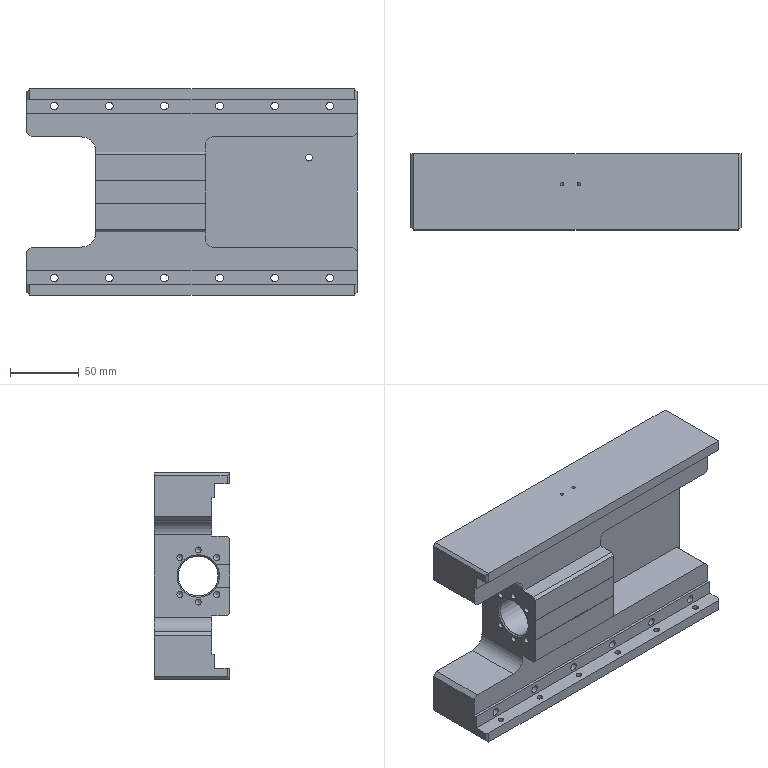CAM job | NX | 3+2 milling, drilling | part box 240 x 55 x 150 mm | stock box 245 x 60 x 155 mm
Tools:
number,name,description,diameter,corner_radius,flute_length,length,flutes
4,D4,平底铣刀-粗,4.0,0.0,25.0,75.0,2
6,D6,平底铣刀-粗,6.0,0.0,25.0,75.0,2
9,D10,平底铣刀-粗,10.0,0.0,35.0,75.0,2
17,D16,平底铣刀-粗,16.0,0.0,50.0,75.0,2
11,D4-J,平底铣刀-精,4.0,0.0,50.0,75.0,2
7,D6-J,平底铣刀-精,6.0,0.0,25.0,75.0,2
10,D10-J,平底铣刀-精,10.0,0.0,35.0,75.0,2
18,D16-J,平底铣刀-精,16.0,0.0,50.0,75.0,2
1,D80R0.8飞刀,圆鼻刀-粗,80.0,0.8,50.0,75.0,2
1,D80R0.8飞刀-J,圆鼻刀-精,80.0,0.8,50.0,75.0,2
2,D6倒角刀,倒角刀,6.0,0.0,3.0,25.0,2
19,D10倒角刀,倒角刀,10.0,0.0,5.0,75.0,2
21,M4X0.7,丝锥,3.3,0.0,35.0,50.0,2
22,M5X0.8,丝锥,4.2,0.0,35.0,50.0,2
23,M6X1.0,丝锥,5.0,0.0,35.0,50.0,2
15,ZT5,钻头,5.0,0.0,35.0,50.0,2
22,ZT5.5,钻头,5.5,0.0,35.0,50.0,2
18,ZT5.8,钻头,5.8,0.0,35.0,50.0,2
13,钻头3.3,Twist Drill 3.3 mm,3.3,0.0,35.0,35.008,2
14,钻头4.2,Twist Drill 4.2 mm,4.2,0.0,41.0,41.738,2
Operations:
program,operation,operation_type,tool,method,geometry_group,spindle_rpm,surface_speed,feed_per_tooth,feed_cut,feed_plunge,cut_length_mm,path_length_mm,cut_time_min,machine_time_min
C,等高往复层切开粗-中_COPY,ZLevelMilling,D16,分层开粗-切深K-步距G,W-C,4000.0,201.062,0.5,4000.0,100.0,13176.223,13478.223,3.294,3.324
C,打点-深0.8_2,Operation,D10倒角刀,NONE,W-C,5000.0,157.08,0.05,500.0,90.0,10.8,251.794,0.0216,0.0457
C,盲锥孔-M5螺纹底孔_2,Operation,钻头4.2,NONE,W-C,2500.0,32.987,0.03,150.0,90.0,87.971,406.136,0.5865,0.6183
C,铣倒角_6,PlanarMilling,D10倒角刀,METHOD,W-C,5000.0,157.08,0.05,500.0,100.0,86.111,1019.558,0.1722,0.2656
C,底壁铣倒角_COPY_1,VolumeBased25DMillingOperation,D10倒角刀,爬面_倒角-切深0-步距G,W-C,5000.0,157.08,0.1,1000.0,100.0,98.812,239.212,0.0988,0.1129
C,C0.3封闭铣廓倒角6X45L_COPY,PlanarMilling,D10倒角刀,爬面_倒角-切深0-步距G,W-C,5000.0,157.08,0.1,1000.0,100.0,45.144,335.469,0.0451,0.0742
C,底壁铣精光侧面-中_COPY,VolumeBased25DMillingOperation,D16-J,侧刃精光-切深K-步距G,W-C,3000.0,150.796,0.1667,1000.0,100.0,1007.169,1368.887,1.007,1.043
B,底壁铣飞面开粗_COPY,VolumeBased25DMillingOperation,D80R0.8飞刀,分层开粗-切深K-步距G,W-B,2800.0,703.696,0.5357,3000.0,100.0,9535.189,12950.012,3.178,3.52
B,底壁铣飞面精光_COPY,VolumeBased25DMillingOperation,D80R0.8飞刀-J,侧刃精光-切深K-步距G,W-B,4000.0,1005.28,0.125,1000.0,100.0,1058.658,1154.658,1.059,1.068
B,型腔铣开粗-中_COPY_1,CavityMilling,D10,分层开粗-切深K-步距G,W-B,8000.0,251.327,0.3125,5000.0,100.0,156407.598,167969.499,31.282,32.886
B,底壁铣精光底面-中_COPY,VolumeBased25DMillingOperation,D10-J,精光步距切深关,W-B,7000.0,175.0,0.0536,1500.0,100.0,3911.458,4582.386,2.608,2.675
B,底壁铣精光底面-中_COPY_1,VolumeBased25DMillingOperation,D10-J,精光步距切深关,W-B,7000.0,175.0,0.0536,1500.0,100.0,1585.376,1695.376,1.057,1.068
B,底壁铣精光侧面-中-选底面_COPY_1,VolumeBased25DMillingOperation,D10-J,侧刃精光-切深K-步距G,W-B,8000.0,251.32,0.0625,1000.0,100.0,712.444,972.215,0.7124,0.7384
B,底壁铣精光侧面-中-选底面_COPY_2,VolumeBased25DMillingOperation,D10-J,侧刃精光-切深K-步距G,W-B,8000.0,251.32,0.0625,1000.0,100.0,904.927,1155.753,0.9049,0.93
B,平面去毛刺6X45L_COPY,SurfaceContour,D6倒角刀,爬面_倒角-切深0-步距G,W-B,6500.0,122.519,0.1154,1500.0,100.0,2590.157,5472.976,1.727,2.015
B,底壁铣倒角_COPY,VolumeBased25DMillingOperation,D6倒角刀,爬面_倒角-切深0-步距G,W-B,6500.0,122.519,0.1154,1500.0,100.0,256.429,1478.093,0.171,0.2931
B,底壁铣精光侧面-中-选底面_COPY,VolumeBased25DMillingOperation,D10-J,侧刃精光-切深K-步距G,W-B,8000.0,251.32,0.0625,1000.0,100.0,516.566,711.587,0.5166,0.5361
A,顶面,FaceMilling,D80R0.8飞刀,侧刃精光-切深K-步距G,W-A,4000.0,1005.31,0.125,1000.0,100.0,1432.0,1468.0,1.432,1.436
A,型腔铣开粗-中_COPY,CavityMilling,D10,分层开粗-切深K-步距G,W-A,6000.0,188.496,0.4167,5000.0,100.0,133321.075,136974.045,26.664,27.235
A,打点-深0.8,Operation,D6倒角刀,NONE,W-A,8000.0,150.796,0.0312,500.0,90.0,41.4,834.905,0.0828,0.1622
A,通孔-M6螺纹底孔,Operation,ZT5,NONE,W-A,2800.0,43.982,0.0625,350.0,90.0,21.502,83.004,0.0614,0.0676
A,盲锥孔-M6螺纹底孔,Operation,ZT5,NONE,W-A,2500.0,39.27,0.03,150.0,90.0,87.511,609.047,0.5834,0.6356
A,盲锥孔-M4螺纹底孔,Operation,钻头3.3,NONE,W-A,3000.0,31.102,0.02,120.0,90.0,12.091,64.183,0.1008,0.106
A,盲锥孔-M5螺纹底孔,Operation,钻头4.2,NONE,W-A,2500.0,32.987,0.03,150.0,90.0,29.324,124.667,0.1955,0.205
A,沉头孔-钻孔0段,Operation,ZT5.5,NONE,W-A,1200.0,20.735,0.0625,150.0,90.0,583.828,1743.786,3.892,4.008
A,通孔-精孔6.0预钻14.8,Operation,ZT5.8,NONE,W-A,2500.0,45.553,0.03,150.0,90.0,17.405,155.817,0.116,0.1299
A,铣孔开粗D6_1,CylinderMilling,D6,NONE,W-A,8000.0,150.796,0.075,1200.0,100.0,7527.378,8826.378,6.273,6.403
A,铣孔精光D6_1,CylinderMilling,D6-J,精光步距切深关,W-A,8000.0,150.796,0.0312,500.0,100.0,1036.978,2341.978,2.074,2.204
A,铣孔开粗D4_1,CylinderMilling,D4,NONE,W-A,8000.0,100.531,0.0375,600.0,100.0,273.984,444.984,0.4566,0.4737
A,仅选体,SurfaceContour,D6倒角刀,METHOD,W-A,8000.0,150.796,0.1875,3000.0,100.0,880.51,916.311,0.2935,0.2971
A,钻倒角_1,Operation,D6倒角刀,METHOD,W-A,8000.0,150.796,0.0312,500.0,0.0,5.2,50.4,0.0104,0.0149
A,铣倒角_1,PlanarMilling,D6倒角刀,METHOD,W-A,8000.0,150.796,0.0312,500.0,100.0,34.274,142.094,0.0685,0.0793
A,铣倒角_2,PlanarMilling,D6倒角刀,METHOD,W-A,8000.0,150.796,0.0375,600.0,100.0,94.776,694.582,0.158,0.2179
A,铣倒角_3,PlanarMilling,D6倒角刀,METHOD,W-A,8000.0,150.796,0.0312,500.0,100.0,19.938,61.138,0.0399,0.044
A,铣倒角_4,PlanarMilling,D6倒角刀,METHOD,W-A,8000.0,150.796,0.0312,500.0,100.0,41.927,203.96,0.0839,0.1001
A,铣倒角_5,PlanarMilling,D6倒角刀,NONE,W-A,8000.0,150.796,0.05,800.0,100.0,483.012,1453,0.6038,0.7008
A,盲锥孔-攻牙M4,Operation,M4X0.7,METHOD,W-A,800.0,8.294,0.0004,0.7,90.0,9.1,58.2,13.0,13.005
A,盲锥孔-攻牙M5,Operation,M5X0.8,METHOD,W-A,500.0,6.597,0.0008,0.8,90.0,22.8,111.62,28.5,28.509
A,盲锥孔-攻牙M6,Operation,M6X1.0,METHOD,W-A,500.0,7.854,0.001,1.0,90.0,70.0,574.026,70.0,70.05
A,通孔-攻牙M6,Operation,M6X1.0,METHOD,W-A,500.0,7.854,0.001,1.0,90.0,17.5,75.0,17.5,17.506
A,铣孔精光D4-J_1,CylinderMilling,D4-J,精光步距切深关,W-A,8000.0,100.531,0.0125,200.0,100.0,102.347,273.347,0.5117,0.5288
A,外形半精_2,VolumeBased25DMillingOperation,D10-J,METHOD,W-A,8000.0,251.327,0.0625,1000.0,100.0,2698.767,3040.796,2.699,2.733